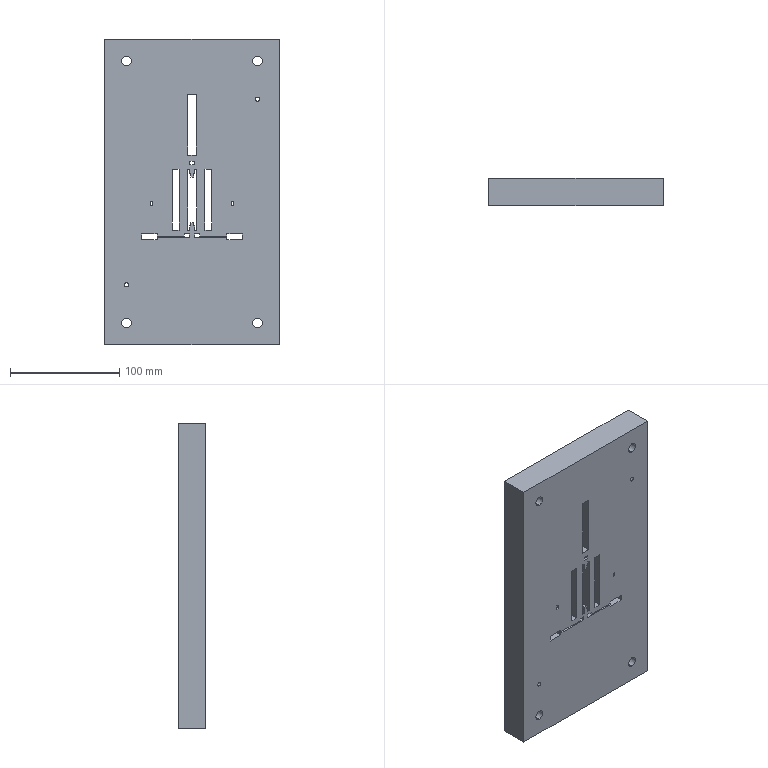Part | SolidWorks | features Cut 5, ICE 2, Extrusion 1, HoleWzd 1 | 1 solid | 147 faces | box 160 x 25 x 280 mm | volume 1024971 mm3 | plane 101 | cylinder 46 | commonest cylinder face diameters 5 x12 3 x8 9 x8 18 x8 4 x4 76.24 x4